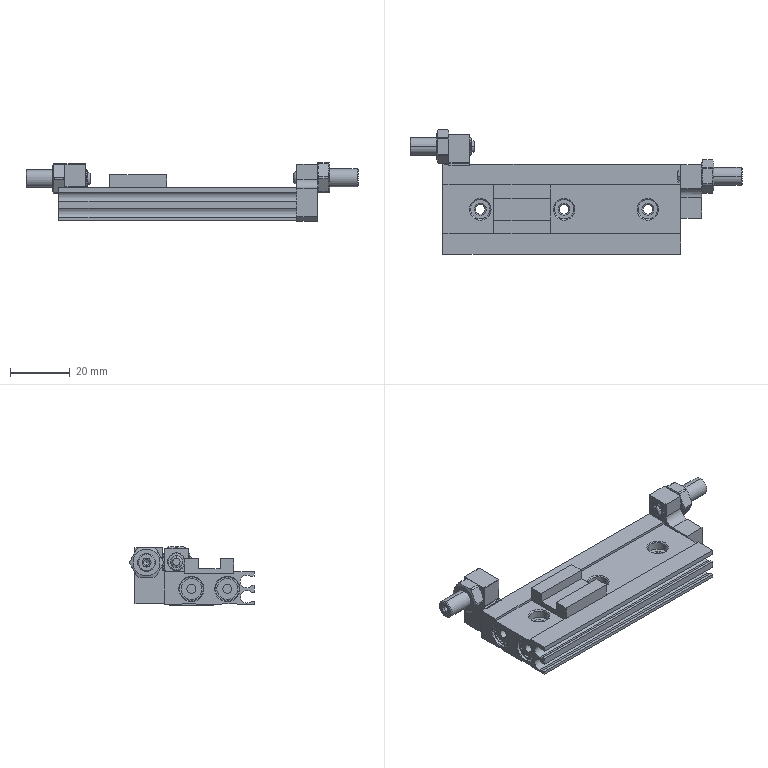Part | STEP file | 11-_HLQ6X40-S-A-0-H-1-body11 | 1 solid | 387 faces | box 111 x 41.6 x 19.5 mm | volume 23196 mm3 | cylinder 135 | plane 134 | cone 98 | spline 20 | commonest cylinder face diameters 3 x17 6 x16 2.013 x12 11.2 x12 1.5 x8 2 x8